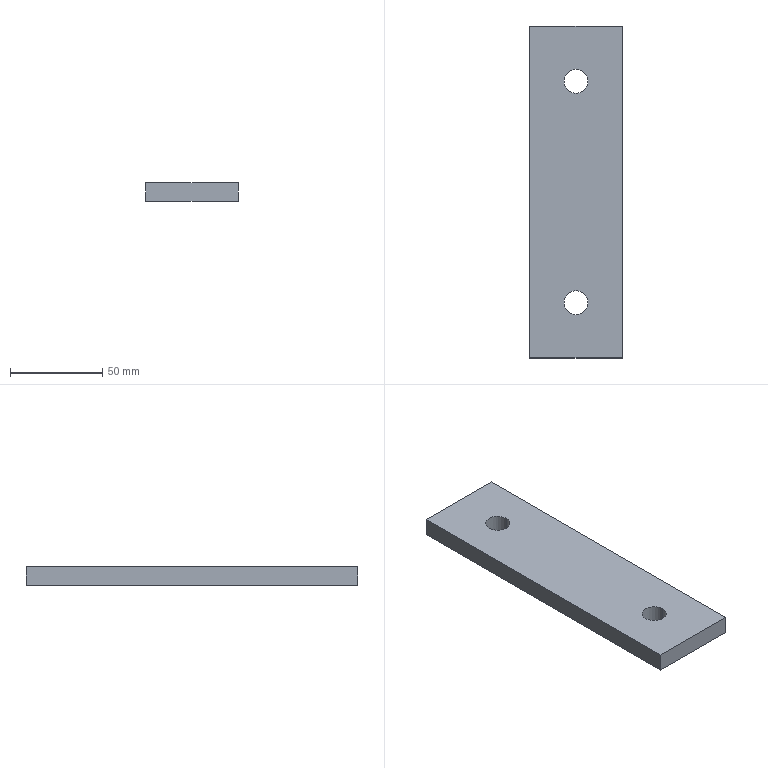Part | SolidWorks | features Extrusion 1, ICE 1 | 1 solid | 10 faces | box 50 x 180 x 10 mm | volume 87345 mm3 | plane 6 | cylinder 4 | commonest cylinder face diameters 13 x4
STEP:
#1=CARTESIAN_POINT('',(18.5,30.,0.));
#2=VERTEX_POINT('',#1);
#3=CARTESIAN_POINT('',(31.5,30.,0.));
#4=VERTEX_POINT('',#3);
#5=CARTESIAN_POINT('',(25.,30.,0.));
#6=DIRECTION('',(0.,0.,1.));
#7=DIRECTION('',(1.,0.,0.));
#8=AXIS2_PLACEMENT_3D('',#5,#6,#7);
#9=CIRCLE('',#8,6.5);
#10=EDGE_CURVE('',#2,#4,#9,.T.);
#11=ORIENTED_EDGE('',*,*,#10,.F.);
#12=CARTESIAN_POINT('',(18.5,30.,10.));
#13=VERTEX_POINT('',#12);
#14=CARTESIAN_POINT('',(18.5,30.,0.));
#15=DIRECTION('',(0.,0.,1.));
#16=VECTOR('',#15,1000.);
#17=LINE('',#14,#16);
#18=EDGE_CURVE('',#2,#13,#17,.T.);
#19=ORIENTED_EDGE('',*,*,#18,.T.);
#20=CARTESIAN_POINT('',(31.5,30.,10.));
#21=VERTEX_POINT('',#20);
#22=CARTESIAN_POINT('',(25.,30.,10.));
#23=DIRECTION('',(0.,0.,1.));
#24=DIRECTION('',(1.,0.,0.));
#25=AXIS2_PLACEMENT_3D('',#22,#23,#24);
#26=CIRCLE('',#25,6.5);
#27=EDGE_CURVE('',#13,#21,#26,.T.);
#28=ORIENTED_EDGE('',*,*,#27,.T.);
#29=CARTESIAN_POINT('',(31.5,30.,0.));
#30=DIRECTION('',(0.,0.,1.));
#31=VECTOR('',#30,1000.);
#32=LINE('',#29,#31);
#33=EDGE_CURVE('',#4,#21,#32,.T.);
#34=ORIENTED_EDGE('',*,*,#33,.F.);
#35=EDGE_LOOP('',(#11,#19,#28,#34));
#36=FACE_OUTER_BOUND('',#35,.T.);
#37=CARTESIAN_POINT('',(25.,30.,0.));
#38=DIRECTION('',(0.,0.,1.));
#39=DIRECTION('',(1.,0.,0.));
#40=AXIS2_PLACEMENT_3D('',#37,#38,#39);
#41=CYLINDRICAL_SURFACE('',#40,6.5);
#42=ADVANCED_FACE('',(#36),#41,.F.);
#43=CARTESIAN_POINT('',(18.5,150.,0.));
#44=VERTEX_POINT('',#43);
#45=CARTESIAN_POINT('',(31.5,150.,0.));
#46=VERTEX_POINT('',#45);
#47=CARTESIAN_POINT('',(25.,150.,0.));
#48=DIRECTION('',(0.,0.,1.));
#49=DIRECTION('',(1.,0.,0.));
#50=AXIS2_PLACEMENT_3D('',#47,#48,#49);
#51=CIRCLE('',#50,6.5);
#52=EDGE_CURVE('',#44,#46,#51,.T.);
#53=ORIENTED_EDGE('',*,*,#52,.F.);
#54=CARTESIAN_POINT('',(18.5,150.,10.));
#55=VERTEX_POINT('',#54);
#56=CARTESIAN_POINT('',(18.5,150.,0.));
#57=DIRECTION('',(0.,0.,1.));
#58=VECTOR('',#57,1000.);
#59=LINE('',#56,#58);
#60=EDGE_CURVE('',#44,#55,#59,.T.);
#61=ORIENTED_EDGE('',*,*,#60,.T.);
#62=CARTESIAN_POINT('',(31.5,150.,10.));
#63=VERTEX_POINT('',#62);
#64=CARTESIAN_POINT('',(25.,150.,10.));
#65=DIRECTION('',(0.,0.,1.));
#66=DIRECTION('',(1.,0.,0.));
#67=AXIS2_PLACEMENT_3D('',#64,#65,#66);
#68=CIRCLE('',#67,6.5);
#69=EDGE_CURVE('',#55,#63,#68,.T.);
#70=ORIENTED_EDGE('',*,*,#69,.T.);
#71=CARTESIAN_POINT('',(31.5,150.,0.));
#72=DIRECTION('',(0.,0.,1.));
#73=VECTOR('',#72,1000.);
#74=LINE('',#71,#73);
#75=EDGE_CURVE('',#46,#63,#74,.T.);
#76=ORIENTED_EDGE('',*,*,#75,.F.);
#77=EDGE_LOOP('',(#53,#61,#70,#76));
#78=FACE_OUTER_BOUND('',#77,.T.);
#79=CARTESIAN_POINT('',(25.,150.,0.));
#80=DIRECTION('',(0.,0.,1.));
#81=DIRECTION('',(1.,0.,0.));
#82=AXIS2_PLACEMENT_3D('',#79,#80,#81);
#83=CYLINDRICAL_SURFACE('',#82,6.5);
#84=ADVANCED_FACE('',(#78),#83,.F.);
#85=CARTESIAN_POINT('',(0.,0.,0.));
#86=VERTEX_POINT('',#85);
#87=CARTESIAN_POINT('',(50.,0.,0.));
#88=VERTEX_POINT('',#87);
#89=CARTESIAN_POINT('',(50.,0.,0.));
#90=DIRECTION('',(1.,0.,0.));
#91=VECTOR('',#90,1000.);
#92=LINE('',#89,#91);
#93=EDGE_CURVE('',#86,#88,#92,.T.);
#94=ORIENTED_EDGE('',*,*,#93,.T.);
#95=CARTESIAN_POINT('',(50.,0.,10.));
#96=VERTEX_POINT('',#95);
#97=CARTESIAN_POINT('',(50.,0.,10.));
#98=DIRECTION('',(0.,0.,-1.));
#99=VECTOR('',#98,1000.);
#100=LINE('',#97,#99);
#101=EDGE_CURVE('',#96,#88,#100,.T.);
#102=ORIENTED_EDGE('',*,*,#101,.F.);
#103=CARTESIAN_POINT('',(0.,0.,10.));
#104=VERTEX_POINT('',#103);
#105=CARTESIAN_POINT('',(50.,0.,10.));
#106=DIRECTION('',(1.,0.,0.));
#107=VECTOR('',#106,1000.);
#108=LINE('',#105,#107);
#109=EDGE_CURVE('',#104,#96,#108,.T.);
#110=ORIENTED_EDGE('',*,*,#109,.F.);
#111=CARTESIAN_POINT('',(0.,0.,10.));
#112=DIRECTION('',(0.,0.,-1.));
#113=VECTOR('',#112,1000.);
#114=LINE('',#111,#113);
#115=EDGE_CURVE('',#104,#86,#114,.T.);
#116=ORIENTED_EDGE('',*,*,#115,.T.);
#117=EDGE_LOOP('',(#94,#102,#110,#116));
#118=FACE_OUTER_BOUND('',#117,.T.);
#119=CARTESIAN_POINT('',(50.,0.,10.));
#120=DIRECTION('',(0.,1.,0.));
#121=DIRECTION('',(0.,0.,1.));
#122=AXIS2_PLACEMENT_3D('',#119,#120,#121);
#123=PLANE('',#122);
#124=ADVANCED_FACE('',(#118),#123,.F.);
#125=CARTESIAN_POINT('',(50.,180.,0.));
#126=VERTEX_POINT('',#125);
#127=CARTESIAN_POINT('',(50.,180.,0.));
#128=DIRECTION('',(0.,1.,0.));
#129=VECTOR('',#128,1000.);
#130=LINE('',#127,#129);
#131=EDGE_CURVE('',#88,#126,#130,.T.);
#132=ORIENTED_EDGE('',*,*,#131,.T.);
#133=CARTESIAN_POINT('',(50.,180.,10.));
#134=VERTEX_POINT('',#133);
#135=CARTESIAN_POINT('',(50.,180.,10.));
#136=DIRECTION('',(0.,0.,-1.));
#137=VECTOR('',#136,1000.);
#138=LINE('',#135,#137);
#139=EDGE_CURVE('',#134,#126,#138,.T.);
#140=ORIENTED_EDGE('',*,*,#139,.F.);
#141=CARTESIAN_POINT('',(50.,180.,10.));
#142=DIRECTION('',(0.,1.,0.));
#143=VECTOR('',#142,1000.);
#144=LINE('',#141,#143);
#145=EDGE_CURVE('',#96,#134,#144,.T.);
#146=ORIENTED_EDGE('',*,*,#145,.F.);
#147=ORIENTED_EDGE('',*,*,#101,.T.);
#148=EDGE_LOOP('',(#132,#140,#146,#147));
#149=FACE_OUTER_BOUND('',#148,.T.);
#150=CARTESIAN_POINT('',(50.,180.,10.));
#151=DIRECTION('',(-1.,0.,0.));
#152=DIRECTION('',(0.,0.,1.));
#153=AXIS2_PLACEMENT_3D('',#150,#151,#152);
#154=PLANE('',#153);
#155=ADVANCED_FACE('',(#149),#154,.F.);
#156=CARTESIAN_POINT('',(0.,180.,0.));
#157=VERTEX_POINT('',#156);
#158=CARTESIAN_POINT('',(0.,180.,0.));
#159=DIRECTION('',(-1.,0.,0.));
#160=VECTOR('',#159,1000.);
#161=LINE('',#158,#160);
#162=EDGE_CURVE('',#126,#157,#161,.T.);
#163=ORIENTED_EDGE('',*,*,#162,.T.);
#164=CARTESIAN_POINT('',(0.,180.,10.));
#165=VERTEX_POINT('',#164);
#166=CARTESIAN_POINT('',(0.,180.,10.));
#167=DIRECTION('',(0.,0.,-1.));
#168=VECTOR('',#167,1000.);
#169=LINE('',#166,#168);
#170=EDGE_CURVE('',#165,#157,#169,.T.);
#171=ORIENTED_EDGE('',*,*,#170,.F.);
#172=CARTESIAN_POINT('',(0.,180.,10.));
#173=DIRECTION('',(-1.,0.,0.));
#174=VECTOR('',#173,1000.);
#175=LINE('',#172,#174);
#176=EDGE_CURVE('',#134,#165,#175,.T.);
#177=ORIENTED_EDGE('',*,*,#176,.F.);
#178=ORIENTED_EDGE('',*,*,#139,.T.);
#179=EDGE_LOOP('',(#163,#171,#177,#178));
#180=FACE_OUTER_BOUND('',#179,.T.);
#181=CARTESIAN_POINT('',(0.,180.,10.));
#182=DIRECTION('',(0.,-1.,0.));
#183=DIRECTION('',(0.,0.,-1.));
#184=AXIS2_PLACEMENT_3D('',#181,#182,#183);
#185=PLANE('',#184);
#186=ADVANCED_FACE('',(#180),#185,.F.);
#187=CARTESIAN_POINT('',(0.,0.,0.));
#188=DIRECTION('',(0.,-1.,0.));
#189=VECTOR('',#188,1000.);
#190=LINE('',#187,#189);
#191=EDGE_CURVE('',#157,#86,#190,.T.);
#192=ORIENTED_EDGE('',*,*,#191,.T.);
#193=ORIENTED_EDGE('',*,*,#115,.F.);
#194=CARTESIAN_POINT('',(0.,0.,10.));
#195=DIRECTION('',(0.,-1.,0.));
#196=VECTOR('',#195,1000.);
#197=LINE('',#194,#196);
#198=EDGE_CURVE('',#165,#104,#197,.T.);
#199=ORIENTED_EDGE('',*,*,#198,.F.);
#200=ORIENTED_EDGE('',*,*,#170,.T.);
#201=EDGE_LOOP('',(#192,#193,#199,#200));
#202=FACE_OUTER_BOUND('',#201,.T.);
#203=CARTESIAN_POINT('',(0.,0.,10.));
#204=DIRECTION('',(1.,0.,0.));
#205=DIRECTION('',(0.,0.,-1.));
#206=AXIS2_PLACEMENT_3D('',#203,#204,#205);
#207=PLANE('',#206);
#208=ADVANCED_FACE('',(#202),#207,.F.);
#209=CARTESIAN_POINT('',(25.,30.,10.));
#210=DIRECTION('',(0.,0.,1.));
#211=DIRECTION('',(1.,0.,0.));
#212=AXIS2_PLACEMENT_3D('',#209,#210,#211);
#213=CIRCLE('',#212,6.5);
#214=EDGE_CURVE('',#21,#13,#213,.T.);
#215=ORIENTED_EDGE('',*,*,#214,.F.);
#216=ORIENTED_EDGE('',*,*,#27,.F.);
#217=EDGE_LOOP('',(#215,#216));
#218=FACE_BOUND('',#217,.T.);
#219=CARTESIAN_POINT('',(25.,150.,10.));
#220=DIRECTION('',(0.,0.,1.));
#221=DIRECTION('',(1.,0.,0.));
#222=AXIS2_PLACEMENT_3D('',#219,#220,#221);
#223=CIRCLE('',#222,6.5);
#224=EDGE_CURVE('',#63,#55,#223,.T.);
#225=ORIENTED_EDGE('',*,*,#224,.F.);
#226=ORIENTED_EDGE('',*,*,#69,.F.);
#227=EDGE_LOOP('',(#225,#226));
#228=FACE_BOUND('',#227,.T.);
#229=ORIENTED_EDGE('',*,*,#109,.T.);
#230=ORIENTED_EDGE('',*,*,#145,.T.);
#231=ORIENTED_EDGE('',*,*,#176,.T.);
#232=ORIENTED_EDGE('',*,*,#198,.T.);
#233=EDGE_LOOP('',(#229,#230,#231,#232));
#234=FACE_OUTER_BOUND('',#233,.T.);
#235=CARTESIAN_POINT('',(0.,0.,10.));
#236=DIRECTION('',(0.,0.,-1.));
#237=DIRECTION('',(-1.,0.,0.));
#238=AXIS2_PLACEMENT_3D('',#235,#236,#237);
#239=PLANE('',#238);
#240=ADVANCED_FACE('',(#218,#228,#234),#239,.F.);
#241=CARTESIAN_POINT('',(25.,30.,0.));
#242=DIRECTION('',(0.,0.,1.));
#243=DIRECTION('',(1.,0.,0.));
#244=AXIS2_PLACEMENT_3D('',#241,#242,#243);
#245=CIRCLE('',#244,6.5);
#246=EDGE_CURVE('',#4,#2,#245,.T.);
#247=ORIENTED_EDGE('',*,*,#246,.T.);
#248=ORIENTED_EDGE('',*,*,#10,.T.);
#249=EDGE_LOOP('',(#247,#248));
#250=FACE_BOUND('',#249,.T.);
#251=CARTESIAN_POINT('',(25.,150.,0.));
#252=DIRECTION('',(0.,0.,1.));
#253=DIRECTION('',(1.,0.,0.));
#254=AXIS2_PLACEMENT_3D('',#251,#252,#253);
#255=CIRCLE('',#254,6.5);
#256=EDGE_CURVE('',#46,#44,#255,.T.);
#257=ORIENTED_EDGE('',*,*,#256,.T.);
#258=ORIENTED_EDGE('',*,*,#52,.T.);
#259=EDGE_LOOP('',(#257,#258));
#260=FACE_BOUND('',#259,.T.);
#261=ORIENTED_EDGE('',*,*,#93,.F.);
#262=ORIENTED_EDGE('',*,*,#191,.F.);
#263=ORIENTED_EDGE('',*,*,#162,.F.);
#264=ORIENTED_EDGE('',*,*,#131,.F.);
#265=EDGE_LOOP('',(#261,#262,#263,#264));
#266=FACE_OUTER_BOUND('',#265,.T.);
#267=CARTESIAN_POINT('',(0.,0.,0.));
#268=DIRECTION('',(0.,0.,-1.));
#269=DIRECTION('',(-1.,0.,0.));
#270=AXIS2_PLACEMENT_3D('',#267,#268,#269);
#271=PLANE('',#270);
#272=ADVANCED_FACE('',(#250,#260,#266),#271,.T.);
#273=ORIENTED_EDGE('',*,*,#60,.F.);
#274=ORIENTED_EDGE('',*,*,#256,.F.);
#275=ORIENTED_EDGE('',*,*,#75,.T.);
#276=ORIENTED_EDGE('',*,*,#224,.T.);
#277=EDGE_LOOP('',(#273,#274,#275,#276));
#278=FACE_OUTER_BOUND('',#277,.T.);
#279=CARTESIAN_POINT('',(25.,150.,0.));
#280=DIRECTION('',(0.,0.,1.));
#281=DIRECTION('',(1.,0.,0.));
#282=AXIS2_PLACEMENT_3D('',#279,#280,#281);
#283=CYLINDRICAL_SURFACE('',#282,6.5);
#284=ADVANCED_FACE('',(#278),#283,.F.);
#285=ORIENTED_EDGE('',*,*,#18,.F.);
#286=ORIENTED_EDGE('',*,*,#246,.F.);
#287=ORIENTED_EDGE('',*,*,#33,.T.);
#288=ORIENTED_EDGE('',*,*,#214,.T.);
#289=EDGE_LOOP('',(#285,#286,#287,#288));
#290=FACE_OUTER_BOUND('',#289,.T.);
#291=CARTESIAN_POINT('',(25.,30.,0.));
#292=DIRECTION('',(0.,0.,1.));
#293=DIRECTION('',(1.,0.,0.));
#294=AXIS2_PLACEMENT_3D('',#291,#292,#293);
#295=CYLINDRICAL_SURFACE('',#294,6.5);
#296=ADVANCED_FACE('',(#290),#295,.F.);
#297=CLOSED_SHELL('',(#42,#84,#124,#155,#186,#208,#240,#272,#284,#296));
#298=MANIFOLD_SOLID_BREP('',#297);
#299=CARTESIAN_POINT('',(0.,0.,0.));
#300=DIRECTION('',(0.,0.,1.));
#301=DIRECTION('',(1.,0.,0.));
#302=AXIS2_PLACEMENT_3D('',#299,#300,#301);
#303=(LENGTH_UNIT()NAMED_UNIT(*)SI_UNIT(.MILLI.,.METRE.));
#304=UNCERTAINTY_MEASURE_WITH_UNIT(LENGTH_MEASURE(0.00001),#303,'','');
#305=(NAMED_UNIT(*)PLANE_ANGLE_UNIT()SI_UNIT($,.RADIAN.));
#306=(NAMED_UNIT(*)SI_UNIT($,.STERADIAN.)SOLID_ANGLE_UNIT());
#307=(GEOMETRIC_REPRESENTATION_CONTEXT(3)GLOBAL_UNCERTAINTY_ASSIGNED_CONTEXT((#304))GLOBAL_UNIT_ASSIGNED_CONTEXT((#303,#305,#306))REPRESENTATION_CONTEXT('',''));
#308=ADVANCED_BREP_SHAPE_REPRESENTATION('',(#298,#302),#307);